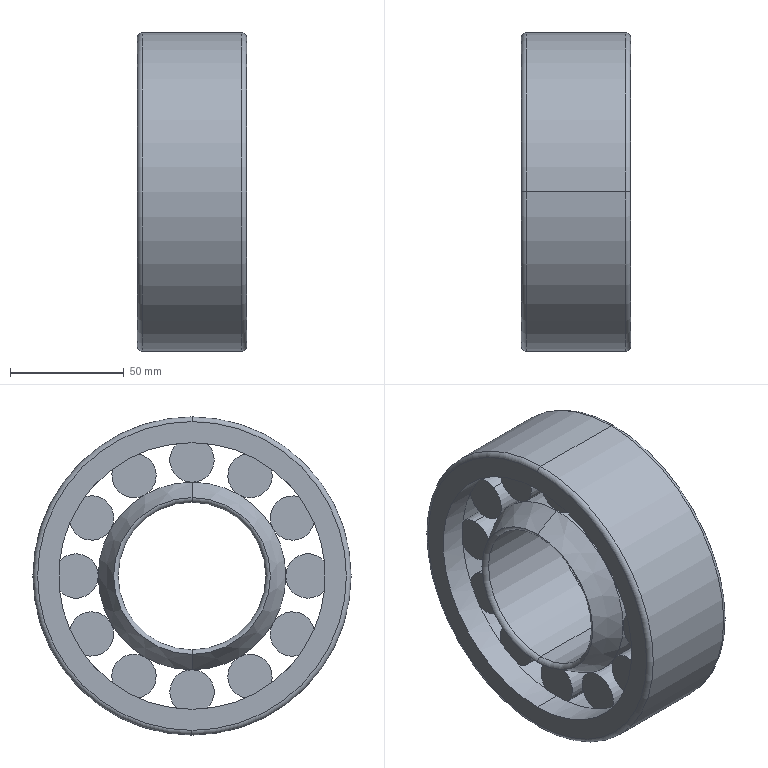Part | SolidWorks | features Revolution 3, CirPattern 1 | 1 solid | 131 faces | box 48 x 140 x 140 mm | volume 368578 mm3 | cylinder 68 | plane 51 | torus 8 | cone 4 | commonest cylinder face diameters 19.5 x36 82.5 x12 121.5 x12 117.3 x4 65 x2 140 x2